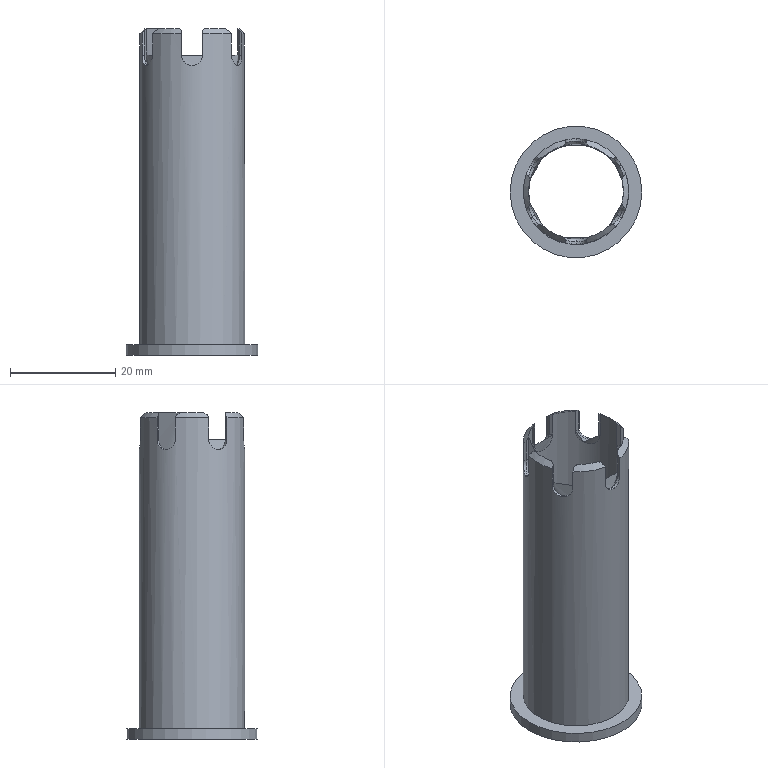Part | NX | features DATUM_CSYS 4, EXTRUDE 3, SKETCH 3, BLEND 2, CHAMFER 2 | 2 solids | 62 faces | box 25 x 25 x 62 mm | volume 14047 mm3 | plane 27 | cylinder 17 | spline 12 | cone 6 | commonest cylinder face diameters 4 x12 18 x3 20 x1 25 x1